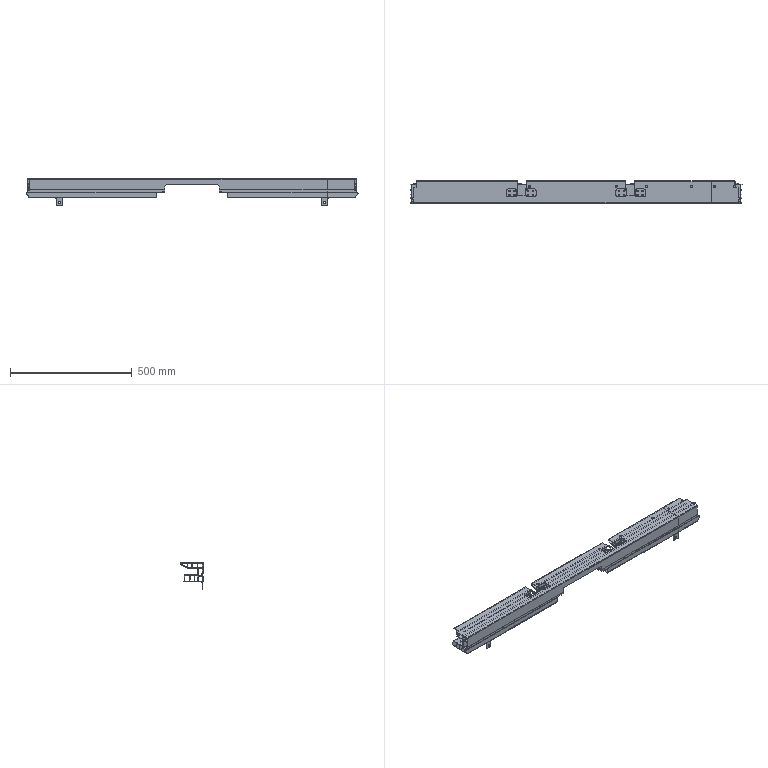NC program | NX | posted with a generic post | part box 1365 x 90.95 x 108.501 mm
Lines 15591 to 16293 of 23380:
(FIXED_CONTOUR_COPY , TOOL : D6)
N31156 T06 M6
N31158 G54
N31160 G17 G0 G90 X-536.513 Y-19.655 B0. C0. S9500 M3
N31162 G43 Z30. H6
N31164 Z-3.359
N31166 G94 G1 Z-8.159 F1000.
N31168 X-536.315 Y-19.457 Z-8.58 F2500.
N31170 X-535.832 Y-18.974 Z-9.536
N31172 X-535.728 Y-18.87 Z-9.73
N31174 X-535.641 Y-18.837 Z-9.891
N31176 X-535.457 Y-18.798 Z-10.212
N31178 X-535.59 Y-18.932 Z-9.981
N31180 X-535.846 Y-19.188 Z-9.51
N31182 X-536.315 Y-19.656 Z-8.576
N31184 X-536.575 Y-19.917 Z-8.023
N31186 X-536.669 Y-20.01 Z-7.818
N31188 X-536.738 Y-20.202 Z-7.664
N31190 X-536.789 Y-20.383 Z-7.549
N31192 X-536.315 Y-19.909 Z-8.572
N31194 X-535.832 Y-19.426 Z-9.539
N31196 X-535.59 Y-19.185 Z-9.982
N31198 X-535.349 Y-18.943 Z-10.392
N31200 X-535.167 Y-18.762 Z-10.649
N31202 X-534.992 Y-18.745 Z-10.887
N31204 X-534.879 Y-18.739 Z-11.039
N31206 X-535.107 Y-18.967 Z-10.728
N31208 X-535.251 Y-19.111 Z-10.528
N31210 X-535.349 Y-19.208 Z-10.389
N31212 X-535.59 Y-19.45 Z-9.983
N31214 X-535.832 Y-19.691 Z-9.538
N31216 X-536.017 Y-19.876 Z-9.168
N31218 X-536.315 Y-20.174 Z-8.564
N31220 X-536.797 Y-20.657 Z-7.521
N31222 X-536.88 Y-20.74 Z-7.338
N31224 X-536.949 Y-21.102 Z-7.178
N31226 X-536.682 Y-20.835 Z-7.76
N31228 X-536.315 Y-20.467 Z-8.554
N31230 X-536.203 Y-20.355 Z-8.785
N31232 X-535.832 Y-19.985 Z-9.538
N31234 X-535.59 Y-19.743 Z-9.986
N31236 X-535.349 Y-19.502 Z-10.388
N31238 X-535.107 Y-19.26 Z-10.729
N31240 X-534.866 Y-19.019 Z-11.056
N31242 X-534.688 Y-18.841 Z-11.269
N31244 X-534.625 Y-18.777 Z-11.349
N31246 X-534.574 Y-18.727 Z-11.406
N31248 X-534.382 Y-18.721 Z-11.611
N31250 X-534.247 Y-18.718 Z-11.745
N31252 X-534.309 Y-18.78 Z-11.682
N31254 X-534.383 Y-18.854 Z-11.61
N31256 X-534.625 Y-19.095 Z-11.344
N31258 X-534.866 Y-19.337 Z-11.056
N31260 X-535.107 Y-19.578 Z-10.731
N31262 X-535.349 Y-19.82 Z-10.39
N31264 X-535.59 Y-20.061 Z-9.988
N31266 X-535.832 Y-20.302 Z-9.536
N31268 X-536.099 Y-20.57 Z-8.992
N31270 X-536.315 Y-20.785 Z-8.541
N31272 X-537. Y-21.47 Z-7.06
N31274 X-537.024 Y-21.668 Z-7.003
N31276 X-537.034 Y-21.829 Z-6.979
N31278 X-536.657 Y-21.453 Z-7.788
N31280 X-536.315 Y-21.11 Z-8.528
N31282 X-536.176 Y-20.972 Z-8.822
N31284 X-535.936 Y-20.731 Z-9.321
N31286 X-535.832 Y-20.628 Z-9.533
N31288 X-535.59 Y-20.386 Z-9.99
N31290 X-535.349 Y-20.145 Z-10.392
N31292 X-535.107 Y-19.903 Z-10.732
N31294 X-534.866 Y-19.662 Z-11.056
N31296 X-534.625 Y-19.42 Z-11.344
N31298 X-534.383 Y-19.179 Z-11.61
N31300 X-534.142 Y-18.938 Z-11.845
N31302 X-533.914 Y-18.71 Z-12.054
N31304 X-533.583 Y-18.705 Z-12.32
N31306 X-533.682 Y-18.804 Z-12.239
N31308 X-533.9 Y-19.022 Z-12.066
N31310 X-534.142 Y-19.264 Z-11.845
N31312 X-534.383 Y-19.505 Z-11.61
N31314 X-534.625 Y-19.747 Z-11.344
N31316 X-534.866 Y-19.988 Z-11.056
N31318 X-535.107 Y-20.23 Z-10.732
N31320 X-535.349 Y-20.471 Z-10.394
N31322 X-535.59 Y-20.712 Z-9.992
N31324 X-535.832 Y-20.954 Z-9.529
N31326 X-536.012 Y-21.135 Z-9.156
N31328 X-536.315 Y-21.437 Z-8.514
N31330 X-536.671 Y-21.793 Z-7.748
N31332 X-537.054 Y-22.176 Z-6.931
N31334 X-537.061 Y-22.509 Z-6.916
N31336 X-536.57 Y-22.019 Z-7.955
N31338 X-536.089 Y-21.538 Z-8.984
N31340 X-535.832 Y-21.28 Z-9.525
N31342 X-535.59 Y-21.039 Z-9.994
N31344 X-535.349 Y-20.797 Z-10.395
N31346 X-535.107 Y-20.556 Z-10.732
N31348 X-534.866 Y-20.314 Z-11.056
N31350 X-534.625 Y-20.073 Z-11.344
N31352 X-534.383 Y-19.831 Z-11.611
N31354 X-534.142 Y-19.59 Z-11.845
N31356 X-533.9 Y-19.349 Z-12.067
N31358 X-533.417 Y-18.866 Z-12.447
N31360 X-533.252 Y-18.7 Z-12.552
N31362 X-532.922 Y-18.696 Z-12.762
N31364 X-533.417 Y-19.192 Z-12.447
N31366 X-533.9 Y-19.675 Z-12.067
N31368 X-534.142 Y-19.916 Z-11.845
N31370 X-534.383 Y-20.158 Z-11.611
N31372 X-534.625 Y-20.399 Z-11.343
N31374 X-534.866 Y-20.64 Z-11.056
N31376 X-535.107 Y-20.882 Z-10.732
N31378 X-535.349 Y-21.123 Z-10.397
N31380 X-535.59 Y-21.365 Z-9.996
N31382 X-535.734 Y-21.508 Z-9.717
N31384 X-535.832 Y-21.606 Z-9.519
N31386 X-536.019 Y-21.793 Z-9.122
N31388 X-536.498 Y-22.272 Z-8.102
N31390 X-537.063 Y-22.837 Z-6.912
N31392 X-537.062 Y-23.162 Z-6.914
N31394 X-536.172 Y-22.272 Z-8.788
N31396 X-535.832 Y-21.932 Z-9.512
N31398 X-535.625 Y-21.725 Z-9.931
N31400 X-535.59 Y-21.691 Z-9.998
N31402 X-535.349 Y-21.449 Z-10.401
N31404 X-535.107 Y-21.208 Z-10.735
N31406 X-534.866 Y-20.967 Z-11.057
N31408 X-534.625 Y-20.725 Z-11.343
N31410 X-534.383 Y-20.484 Z-11.611
N31412 X-534.142 Y-20.242 Z-11.845
N31414 X-533.9 Y-20.001 Z-12.067
N31416 X-533.417 Y-19.518 Z-12.447
N31418 X-532.935 Y-19.035 Z-12.754
N31420 X-532.693 Y-18.794 Z-12.894
N31422 X-532.591 Y-18.692 Z-12.949
N31424 X-532.451 Y-18.689 Z-13.021
N31426 X-532.446 Z-13.025
N31428 X-532.39 Y-18.685 Z-12.995
N31430 X-532.26 Y-18.686 Z-12.925
N31432 X-532.448 Y-18.874 Z-13.023
N31434 X-532.693 Y-19.12 Z-12.893
N31436 X-532.935 Y-19.361 Z-12.754
N31438 X-533.417 Y-19.844 Z-12.447
N31440 X-533.9 Y-20.327 Z-12.067
N31442 X-534.142 Y-20.568 Z-11.845
N31444 X-534.383 Y-20.809 Z-11.611
N31446 X-534.625 Y-21.051 Z-11.345
N31448 X-534.866 Y-21.292 Z-11.06
N31450 X-535.107 Y-21.534 Z-10.741
N31452 X-535.349 Y-21.775 Z-10.409
N31454 X-535.515 Y-21.942 Z-10.133
N31456 X-535.59 Y-22.017 Z-9.993
N31458 X-535.839 Y-22.265 Z-9.489
N31460 X-537.061 Y-23.488 Z-6.916
N31462 Y-23.604 Z-6.917
N31464 X-537.053 Y-23.805 Z-6.936
N31466 X-535.832 Y-22.584 Z-9.502
N31468 X-535.59 Y-22.342 Z-9.986
N31470 X-535.406 Y-22.158 Z-10.329
N31472 X-535.349 Y-22.101 Z-10.424
N31474 X-535.175 Y-21.926 Z-10.659
N31476 X-535.107 Y-21.859 Z-10.753
N31478 X-535.041 Y-21.793 Z-10.835
N31480 X-534.866 Y-21.618 Z-11.066
N31482 X-534.625 Y-21.376 Z-11.348
N31484 X-534.383 Y-21.135 Z-11.613
N31486 X-534.142 Y-20.894 Z-11.845
N31488 X-533.9 Y-20.652 Z-12.067
N31490 X-533.417 Y-20.169 Z-12.447
N31492 X-532.935 Y-19.686 Z-12.754
N31494 X-532.694 Y-19.445 Z-12.894
N31496 X-532.452 Y-19.204 Z-13.024
N31498 X-532.209 Y-18.961 Z-12.893
N31500 X-531.969 Y-18.721 Z-12.754
N31502 X-531.938 Y-18.69 Z-12.735
N31504 X-531.619 Y-18.695 Z-12.532
N31506 X-531.969 Y-19.045 Z-12.754
N31508 X-532.21 Y-19.286 Z-12.894
N31510 X-532.452 Y-19.529 Z-13.024
N31512 X-532.693 Y-19.77 Z-12.894
N31514 X-532.935 Y-20.011 Z-12.754
N31516 X-533.417 Y-20.494 Z-12.447
N31518 X-533.9 Y-20.977 Z-12.068
N31520 X-534.142 Y-21.218 Z-11.847
N31522 X-534.383 Y-21.459 Z-11.616
N31524 X-534.625 Y-21.701 Z-11.353
N31526 X-534.717 Y-21.793 Z-11.246
N31528 X-534.866 Y-21.942 Z-11.085
N31530 X-535.107 Y-22.184 Z-10.78
N31532 X-535.196 Y-22.272 Z-10.657
N31534 X-535.349 Y-22.425 Z-10.432
N31536 X-535.59 Y-22.667 Z-9.985
N31538 X-535.832 Y-22.908 Z-9.501
N31540 X-536.797 Y-23.874 Z-7.474
N31542 X-537.04 Y-24.116 Z-6.969
N31544 X-537.013 Y-24.412 Z-7.035
N31546 X-536.79 Y-24.189 Z-7.495
N31548 X-536.31 Y-23.71 Z-8.496
N31550 X-535.831 Y-23.231 Z-9.502
N31552 X-535.59 Y-22.99 Z-9.985
N31554 X-535.349 Y-22.749 Z-10.432
N31556 X-535.107 Y-22.507 Z-10.787
N31558 X-534.866 Y-22.266 Z-11.118
N31560 X-534.625 Y-22.024 Z-11.379
N31562 X-534.393 Y-21.793 Z-11.609
N31564 X-534.142 Y-21.541 Z-11.85
N31566 X-533.9 Y-21.3 Z-12.069
N31568 X-533.417 Y-20.817 Z-12.447
N31570 X-532.935 Y-20.334 Z-12.754
N31572 X-532.693 Y-20.093 Z-12.894
N31574 X-532.452 Y-19.852 Z-13.024
N31576 X-532.21 Y-19.61 Z-12.894
N31578 X-531.969 Y-19.369 Z-12.754
N31580 X-531.486 Y-18.886 Z-12.447
N31582 X-531.301 Y-18.701 Z-12.305
N31584 X-531.003 Y-18.707 Z-12.066
N31586 X-530.985 Z-12.049
N31588 X-531.003 Y-18.726 Z-12.066
N31590 X-531.486 Y-19.209 Z-12.447
N31592 X-531.969 Y-19.692 Z-12.754
N31594 X-532.21 Y-19.933 Z-12.894
N31596 X-532.451 Y-20.174 Z-13.023
N31598 X-532.693 Y-20.416 Z-12.894
N31600 X-532.935 Y-20.657 Z-12.753
N31602 X-533.417 Y-21.14 Z-12.448
N31604 X-533.9 Y-21.623 Z-12.073
N31606 X-534.07 Y-21.793 Z-11.919
N31608 X-534.383 Y-22.106 Z-11.652
N31610 X-534.55 Y-22.272 Z-11.487
N31612 X-534.625 Y-22.347 Z-11.405
N31614 X-534.866 Y-22.589 Z-11.118
N31616 X-535.107 Y-22.83 Z-10.787
N31618 X-535.349 Y-23.072 Z-10.432
N31620 X-535.59 Y-23.313 Z-9.985
N31622 X-535.832 Y-23.554 Z-9.502
N31624 X-536.797 Y-24.52 Z-7.488
N31626 X-536.978 Y-24.701 Z-7.116
N31628 X-536.936 Y-24.98 Z-7.218
N31630 X-536.797 Y-24.841 Z-7.5
N31632 X-535.832 Y-23.876 Z-9.505
N31634 X-535.59 Y-23.634 Z-9.986
N31636 X-535.349 Y-23.393 Z-10.432
N31638 X-535.107 Y-23.151 Z-10.787
N31640 X-534.866 Y-22.91 Z-11.118
N31642 X-534.625 Y-22.669 Z-11.405
N31644 X-534.383 Y-22.427 Z-11.667
N31646 X-534.228 Y-22.272 Z-11.817
N31648 X-534.138 Y-22.182 Z-11.896
N31650 Z-11.887
N31652 X-534.028 Y-22.072 Z-11.976
N31654 X-533.9 Y-21.944 Z-12.085
N31656 X-533.749 Y-21.793 Z-12.194
N31658 X-533.417 Y-21.461 Z-12.451
N31660 X-532.935 Y-20.979 Z-12.754
N31662 X-532.693 Y-20.737 Z-12.893
N31664 X-532.45 Y-20.495 Z-13.022
N31666 X-532.21 Y-20.254 Z-12.894
N31668 X-531.969 Y-20.013 Z-12.754
N31670 X-531.486 Y-19.53 Z-12.447
N31672 X-531.003 Y-19.047 Z-12.066
N31674 X-530.819 Y-18.863 Z-11.897
N31676 X-530.762 Y-18.806 Z-11.847
N31678 X-530.671 Y-18.715 Z-11.76
N31680 X-530.494 Y-18.72 Z-11.581
N31682 X-530.359 Y-18.724 Z-11.437
N31684 X-530.429 Y-18.794 Z-11.509
N31686 X-530.52 Y-18.886 Z-11.61
N31688 X-530.762 Y-19.127 Z-11.845
N31690 X-531.003 Y-19.368 Z-12.066
N31692 X-531.486 Y-19.851 Z-12.447
N31694 X-531.969 Y-20.334 Z-12.753
N31696 X-532.21 Y-20.575 Z-12.893
N31698 X-532.45 Y-20.815 Z-13.021
N31700 X-532.694 Y-21.059 Z-12.895
N31702 X-532.935 Y-21.3 Z-12.756
N31704 X-533.417 Y-21.783 Z-12.455
N31706 X-533.693 Y-22.058 Z-12.255
N31708 X-533.726 Y-22.091 Z-12.233
N31710 X-533.742 Y-22.108 Z-12.221
N31712 X-533.776 Y-22.141 Z-12.2
N31714 X-533.816 Y-22.181 Z-12.173
N31716 X-533.907 Y-22.272 Z-12.112
N31718 X-534.106 Y-22.471 Z-11.935
N31720 X-534.383 Y-22.748 Z-11.667
N31722 X-534.625 Y-22.99 Z-11.405
N31724 X-534.866 Y-23.231 Z-11.119
N31726 X-535.107 Y-23.473 Z-10.787
N31728 X-535.353 Y-23.718 Z-10.425
N31730 X-535.59 Y-23.956 Z-9.991
N31732 X-535.832 Y-24.197 Z-9.51
N31734 X-536.797 Y-25.163 Z-7.515
N31736 X-536.886 Y-25.251 Z-7.337
N31738 X-536.861 Y-25.378 Z-7.396
N31740 X-536.829 Y-25.511 Z-7.472
N31742 X-536.797 Y-25.479 Z-7.534
N31744 X-536.466 Y-25.148 Z-8.212
N31746 X-536.315 Y-24.996 Z-8.526
N31748 X-535.832 Y-24.513 Z-9.516
N31750 X-535.723 Y-24.405 Z-9.726
N31752 X-535.59 Y-24.272 Z-9.995
N31754 X-535.349 Y-24.03 Z-10.419
N31756 X-535.242 Y-23.923 Z-10.573
N31758 X-535.107 Y-23.789 Z-10.781
N31760 X-535.029 Y-23.71 Z-10.895
N31762 X-534.866 Y-23.547 Z-11.118
N31764 X-534.625 Y-23.306 Z-11.405
N31766 X-534.383 Y-23.065 Z-11.667
N31768 X-534.142 Y-22.823 Z-11.901
N31770 X-533.9 Y-22.582 Z-12.118
N31772 X-533.591 Y-22.272 Z-12.36
N31774 X-533.452 Y-22.134 Z-12.45
N31776 X-533.417 Y-22.099 Z-12.473
N31778 X-533.351 Y-22.033 Z-12.51
N31780 X-533.112 Y-21.793 Z-12.651
N31782 X-532.935 Y-21.616 Z-12.762
N31784 X-532.694 Y-21.376 Z-12.898
N31786 X-532.453 Y-21.134 Z-13.023
N31788 X-532.21 Y-20.891 Z-12.893
N31790 X-531.969 Y-20.65 Z-12.753
N31792 X-531.486 Y-20.167 Z-12.447
N31794 X-531.003 Y-19.685 Z-12.066
N31796 X-530.762 Y-19.443 Z-11.844
N31798 X-530.52 Y-19.202 Z-11.61
N31800 X-530.279 Y-18.96 Z-11.344
N31802 X-530.055 Y-18.737 Z-11.077
N31804 X-529.905 Y-18.745 Z-10.878
N31806 X-529.778 Y-18.757 Z-10.707
N31808 X-529.878 Y-18.857 Z-10.836
N31810 X-530.037 Y-19.016 Z-11.056
N31812 X-530.279 Y-19.258 Z-11.344
N31814 X-530.52 Y-19.499 Z-11.61
N31816 X-530.762 Y-19.741 Z-11.844
N31818 X-531.003 Y-19.982 Z-12.067
N31820 X-531.486 Y-20.465 Z-12.447
N31822 X-531.969 Y-20.948 Z-12.754
N31824 X-532.21 Y-21.189 Z-12.895
N31826 X-532.454 Y-21.433 Z-13.026
N31828 X-532.694 Y-21.673 Z-12.902
N31830 X-532.814 Y-21.793 Z-12.835
N31832 X-532.935 Y-21.913 Z-12.771
N31834 X-533.113 Y-22.092 Z-12.668
N31836 X-533.293 Y-22.272 Z-12.572
N31838 X-533.417 Y-22.396 Z-12.493
N31840 X-533.659 Y-22.638 Z-12.308
N31842 X-533.9 Y-22.879 Z-12.118
N31844 X-534.142 Y-23.121 Z-11.901
N31846 X-534.383 Y-23.362 Z-11.667
N31848 X-534.625 Y-23.603 Z-11.405
N31850 X-534.731 Y-23.71 Z-11.279
N31852 X-534.798 Y-23.777 Z-11.189
N31854 X-534.821 Y-23.8 Z-11.163
N31856 X-534.866 Y-23.845 Z-11.106
N31858 X-534.981 Y-23.96 Z-10.937
N31860 X-535.107 Y-24.086 Z-10.758
N31862 X-535.142 Y-24.121 Z-10.705
N31864 X-535.349 Y-24.328 Z-10.408
N31866 X-535.59 Y-24.569 Z-9.993
N31868 X-535.784 Y-24.763 Z-9.611
N31870 X-535.832 Y-24.811 Z-9.521
N31872 X-536.169 Y-25.148 Z-8.832
N31874 X-536.315 Y-25.293 Z-8.538
N31876 X-536.762 Y-25.741 Z-7.624
N31878 X-536.747 Y-25.792 Z-7.659
N31880 X-536.687 Y-25.958 Z-7.793
N31882 X-536.315 Y-25.586 Z-8.55
N31884 X-535.832 Y-25.103 Z-9.525
N31886 X-535.686 Y-24.957 Z-9.803
N31888 X-535.59 Y-24.862 Z-9.991
N31890 X-535.526 Y-24.797 Z-10.098
N31892 X-535.349 Y-24.62 Z-10.4
N31894 X-535.107 Y-24.379 Z-10.745
N31896 X-534.883 Y-24.155 Z-11.053
N31898 X-534.866 Y-24.137 Z-11.078
N31900 X-534.723 Y-23.994 Z-11.26
N31902 X-534.652 Y-23.923 Z-11.342
N31904 X-534.562 Y-23.834 Z-11.461
N31906 X-534.439 Y-23.71 Z-11.607
N31908 X-534.383 Y-23.655 Z-11.667
N31910 X-534.142 Y-23.413 Z-11.901
N31912 X-533.9 Y-23.172 Z-12.118
N31914 X-533.48 Y-22.752 Z-12.447
N31916 X-533.417 Y-22.689 Z-12.495
N31918 X-533.001 Y-22.272 Z-12.758
N31920 X-532.935 Y-22.206 Z-12.794
N31922 X-532.821 Y-22.092 Z-12.847
N31924 X-532.695 Y-21.966 Z-12.912
N31926 X-532.522 Y-21.793 Z-12.995
N31928 X-532.454 Y-21.725 Z-13.03
N31930 X-532.21 Y-21.482 Z-12.898
N31932 X-531.969 Y-21.24 Z-12.756
N31934 X-531.486 Y-20.757 Z-12.447
N31936 X-531.003 Y-20.275 Z-12.067
N31938 X-530.762 Y-20.033 Z-11.844
N31940 X-530.52 Y-19.792 Z-11.61
N31942 X-530.279 Y-19.55 Z-11.343
N31944 X-530.037 Y-19.309 Z-11.056
N31946 X-529.906 Y-19.178 Z-10.878
N31948 X-529.746 Y-19.017 Z-10.654
N31950 X-529.646 Y-18.918 Z-10.512
N31952 X-529.585 Y-18.857 Z-10.428
N31954 X-529.514 Y-18.785 Z-10.311
N31956 X-529.313 Y-18.826 Z-9.987
N31958 X-529.276 Y-18.834 Z-9.918
N31960 X-529.313 Y-18.872 Z-9.983
N31962 X-529.359 Y-18.918 Z-10.056
N31964 X-529.555 Y-19.113 Z-10.384
N31966 X-529.81 Y-19.369 Z-10.748
N31968 X-530.037 Y-19.596 Z-11.056
N31970 X-530.279 Y-19.837 Z-11.343
N31972 X-530.52 Y-20.079 Z-11.61
N31974 X-530.762 Y-20.32 Z-11.844
N31976 X-531.003 Y-20.562 Z-12.067
N31978 X-531.486 Y-21.045 Z-12.448
N31980 X-531.969 Y-21.527 Z-12.759
N31982 X-532.235 Y-21.793 Z-12.915
N31984 X-532.455 Y-22.013 Z-13.041
N31986 X-532.534 Y-22.092 Z-13.003
N31988 X-532.714 Y-22.272 Z-12.923
N31990 X-532.935 Y-22.493 Z-12.801
N31992 X-533.417 Y-22.976 Z-12.495
N31994 X-533.9 Y-23.459 Z-12.118
N31996 X-534.152 Y-23.71 Z-11.891
N31998 X-534.188 Y-23.746 Z-11.846
N32000 X-534.228 Y-23.787 Z-11.803
N32002 X-534.306 Y-23.864 Z-11.727
N32004 X-534.383 Y-23.942 Z-11.645
N32006 X-534.466 Y-24.025 Z-11.547
N32008 X-534.507 Y-24.066 Z-11.492
N32010 X-534.631 Y-24.189 Z-11.35
N32012 X-534.866 Y-24.425 Z-11.067
N32014 X-535.107 Y-24.666 Z-10.737
N32016 X-535.349 Y-24.907 Z-10.393
N32018 X-535.429 Y-24.988 Z-10.255
N32020 X-535.59 Y-25.148 Z-9.99
N32022 X-535.75 Y-25.309 Z-9.681
N32024 X-535.832 Y-25.39 Z-9.529
N32026 X-536.191 Y-25.75 Z-8.802
N32028 X-536.315 Y-25.873 Z-8.559
N32030 X-536.604 Y-26.163 Z-7.975
N32032 X-536.552 Y-26.286 Z-8.092
N32034 X-536.509 Y-26.36 Z-8.181
N32036 X-536.045 Y-25.895 Z-9.1
N32038 X-535.832 Y-25.682 Z-9.532
N32040 X-535.653 Y-25.503 Z-9.867
N32042 X-535.59 Y-25.441 Z-9.987
N32044 X-535.349 Y-25.199 Z-10.387
N32046 X-535.107 Y-24.958 Z-10.732
N32048 X-535.01 Y-24.861 Z-10.865
N32050 X-534.866 Y-24.717 Z-11.06
N32052 X-534.625 Y-24.475 Z-11.351
N32054 X-534.383 Y-24.234 Z-11.621
N32056 X-534.339 Y-24.189 Z-11.664
N32058 X-534.208 Y-24.058 Z-11.803
N32060 X-534.002 Y-23.852 Z-12.007
N32062 X-533.9 Y-23.751 Z-12.115
N32064 X-533.877 Y-23.728 Z-12.136
N32066 X-533.417 Y-23.268 Z-12.495
N32068 X-532.935 Y-22.785 Z-12.801
N32070 X-532.693 Y-22.544 Z-12.934
N32072 X-532.453 Y-22.303 Z-13.054
N32074 X-532.398 Y-22.248 Z-13.023
N32076 X-532.21 Y-22.061 Z-12.914
N32078 X-532.076 Y-21.926 Z-12.831
N32080 X-531.943 Y-21.793 Z-12.746
N32082 X-531.486 Y-21.337 Z-12.449
N32084 X-531.003 Y-20.854 Z-12.067
N32086 X-530.762 Y-20.612 Z-11.845
N32088 X-530.52 Y-20.371 Z-11.61
N32090 X-530.279 Y-20.129 Z-11.343
N32092 X-530.037 Y-19.888 Z-11.056
N32094 X-529.796 Y-19.647 Z-10.729
N32096 X-529.555 Y-19.405 Z-10.387
N32098 X-529.313 Y-19.164 Z-9.979
N32100 X-529.061 Y-18.912 Z-9.522
N32102 X-528.909 Y-18.973 Z-9.227
N32104 X-528.864 Y-19.018 Z-9.139
N32106 X-529.072 Y-19.226 Z-9.537
N32108 X-529.313 Y-19.468 Z-9.979
N32110 X-529.555 Y-19.709 Z-10.387
N32112 X-529.796 Y-19.951 Z-10.729
N32114 X-530.037 Y-20.192 Z-11.056
N32116 X-530.279 Y-20.433 Z-11.343
N32118 X-530.52 Y-20.675 Z-11.611
N32120 X-530.762 Y-20.916 Z-11.845
N32122 X-531.003 Y-21.158 Z-12.068
N32124 X-531.486 Y-21.641 Z-12.453
N32126 X-531.639 Y-21.793 Z-12.552
N32128 X-531.786 Y-21.94 Z-12.656
N32130 X-531.803 Y-21.958 Z-12.669
N32132 X-531.934 Y-22.088 Z-12.757
N32134 X-532.01 Y-22.164 Z-12.809
N32136 X-532.118 Y-22.272 Z-12.879
N32138 X-532.34 Y-22.494 Z-12.998
N32140 X-532.452 Y-22.607 Z-13.054
N32142 X-532.693 Y-22.848 Z-12.934
N32144 X-532.935 Y-23.089 Z-12.801
N32146 X-533.417 Y-23.572 Z-12.494
N32148 X-533.574 Y-23.728 Z-12.373
N32150 X-533.601 Y-23.755 Z-12.346
N32152 X-533.646 Y-23.8 Z-12.309
N32154 X-533.698 Y-23.852 Z-12.259
N32156 X-533.761 Y-23.915 Z-12.205
N32158 X-533.83 Y-23.985 Z-12.144
N32160 X-533.9 Y-24.055 Z-12.084
N32162 X-534.035 Y-24.189 Z-11.952
N32164 X-534.142 Y-24.296 Z-11.853
N32166 X-534.383 Y-24.538 Z-11.616
N32168 X-534.625 Y-24.779 Z-11.345
N32170 X-534.866 Y-25.02 Z-11.057
N32172 X-535.107 Y-25.262 Z-10.728
N32174 X-535.349 Y-25.503 Z-10.386
N32176 X-535.59 Y-25.745 Z-9.984
N32178 X-535.711 Y-25.866 Z-9.755
N32180 X-535.832 Y-25.986 Z-9.532
N32182 X-535.952 Y-26.106 Z-9.292
N32184 X-536.399 Y-26.553 Z-8.416
N32186 X-536.371 Y-26.602 Z-8.475
N32188 X-536.262 Y-26.734 Z-8.698
N32190 X-536.113 Y-26.585 Z-8.983
N32192 X-535.832 Y-26.304 Z-9.533
N32194 X-535.59 Y-26.063 Z-9.981
N32196 X-535.444 Y-25.917 Z-10.228
N32198 X-535.349 Y-25.821 Z-10.386
N32200 X-535.107 Y-25.58 Z-10.729
N32202 X-534.866 Y-25.338 Z-11.056
N32204 X-534.625 Y-25.097 Z-11.343
N32206 X-534.383 Y-24.856 Z-11.613
N32208 X-534.142 Y-24.614 Z-11.848
N32210 X-533.9 Y-24.373 Z-12.073
N32212 X-533.717 Y-24.189 Z-12.22
N32214 X-533.417 Y-23.89 Z-12.473
N32216 X-533.238 Y-23.71 Z-12.607
N32218 X-532.935 Y-23.407 Z-12.8
N32220 X-532.876 Y-23.348 Z-12.831
N32222 X-532.693 Y-23.166 Z-12.934
N32224 X-532.452 Y-22.924 Z-13.054
N32226 X-532.21 Y-22.683 Z-12.933
N32228 X-531.969 Y-22.441 Z-12.799
N32230 X-531.8 Y-22.272 Z-12.691
N32232 X-531.696 Y-22.168 Z-12.614
N32234 X-531.644 Y-22.116 Z-12.58
N32236 X-531.568 Y-22.04 Z-12.521
N32238 X-531.486 Y-21.958 Z-12.464
N32240 X-531.321 Y-21.793 Z-12.325
N32242 X-531.003 Y-21.476 Z-12.071
N32244 X-530.762 Y-21.234 Z-11.847
N32246 X-530.52 Y-20.993 Z-11.612
N32248 X-530.279 Y-20.751 Z-11.343
N32250 X-530.037 Y-20.51 Z-11.056
N32252 X-529.796 Y-20.268 Z-10.729
N32254 X-529.555 Y-20.027 Z-10.386
N32256 X-529.313 Y-19.786 Z-9.98
N32258 X-529.072 Y-19.544 Z-9.533
N32260 X-528.89 Y-19.362 Z-9.18
N32262 X-528.708 Y-19.181 Z-8.831
N32264 X-528.661 Y-19.23 Z-8.737
N32266 X-528.565 Y-19.357 Z-8.543
N32268 X-529.072 Y-19.864 Z-9.532
N32270 X-529.313 Y-20.105 Z-9.983
N32272 X-529.397 Y-20.189 Z-10.124
N32274 X-529.555 Y-20.347 Z-10.386
N32276 X-529.796 Y-20.588 Z-10.728
N32278 X-530.037 Y-20.83 Z-11.056
N32280 X-530.279 Y-21.071 Z-11.344
N32282 X-530.52 Y-21.312 Z-11.614
N32284 X-530.762 Y-21.554 Z-11.85
N32286 X-531.003 Y-21.795 Z-12.075
N32288 X-531.367 Y-22.159 Z-12.386
N32290 X-531.486 Y-22.278 Z-12.491
N32292 X-531.969 Y-22.761 Z-12.801
N32294 X-532.21 Y-23.002 Z-12.934
N32296 X-532.452 Y-23.244 Z-13.054
N32298 X-532.693 Y-23.485 Z-12.93
N32300 X-532.769 Y-23.561 Z-12.887
N32302 X-532.918 Y-23.71 Z-12.808
N32304 X-532.935 Y-23.727 Z-12.797
N32306 X-533.158 Y-23.95 Z-12.633
N32308 X-533.417 Y-24.209 Z-12.455
N32310 X-533.9 Y-24.692 Z-12.069
N32312 X-534.142 Y-24.934 Z-11.846
N32314 X-534.383 Y-25.175 Z-11.611
N32316 X-534.625 Y-25.417 Z-11.343
N32318 X-534.866 Y-25.658 Z-11.056
N32320 X-535.107 Y-25.899 Z-10.729
N32322 X-535.349 Y-26.141 Z-10.387
N32324 X-535.59 Y-26.382 Z-9.98
N32326 X-535.838 Y-26.63 Z-9.523
N32328 X-536.108 Y-26.9 Z-9.004
N32330 X-535.961 Y-27.042 Z-9.296
N32332 X-535.938 Y-27.051 Z-9.34
N32334 X-535.832 Y-26.945 Z-9.54
N32336 X-535.59 Y-26.704 Z-9.979
N32338 X-535.349 Y-26.462 Z-10.387
N32340 X-535.107 Y-26.221 Z-10.729
N32342 X-534.866 Y-25.98 Z-11.056
N32344 X-534.625 Y-25.738 Z-11.343
N32346 X-534.383 Y-25.497 Z-11.611
N32348 X-534.142 Y-25.255 Z-11.845
N32350 X-533.9 Y-25.014 Z-12.068
N32352 X-533.417 Y-24.531 Z-12.451
N32354 X-533.076 Y-24.189 Z-12.671
N32356 X-532.935 Y-24.048 Z-12.768
N32358 X-532.693 Y-23.807 Z-12.92
N32360 X-532.597 Y-23.71 Z-12.974
N32362 X-532.452 Y-23.565 Z-13.048
N32364 X-532.21 Y-23.324 Z-12.932
N32366 X-531.969 Y-23.082 Z-12.801
N32368 X-531.486 Y-22.6 Z-12.494
N32370 X-531.159 Y-22.272 Z-12.24
N32372 X-531.003 Y-22.117 Z-12.099
N32374 X-530.961 Y-22.075 Z-12.057
N32376 X-530.947 Y-22.061 Z-12.041
N32378 X-530.734 Y-21.848 Z-11.832
N32380 X-530.68 Y-21.793 Z-11.774
N32382 X-530.52 Y-21.634 Z-11.618
N32384 X-530.279 Y-21.392 Z-11.347
N32386 X-530.037 Y-21.151 Z-11.058
N32388 X-529.932 Y-21.045 Z-10.916
N32390 X-529.771 Y-20.884 Z-10.694
N32392 X-529.555 Y-20.668 Z-10.386
N32394 X-529.313 Y-20.427 Z-9.986
N32396 X-529.072 Y-20.185 Z-9.532
N32398 X-528.891 Y-20.005 Z-9.167
N32400 X-528.565 Y-19.678 Z-8.526
N32402 X-528.443 Y-19.556 Z-8.284
N32404 X-528.347 Y-19.72 Z-8.082
N32406 X-528.329 Y-19.764 Z-8.041
N32408 X-528.441 Y-19.876 Z-8.263
N32410 X-528.589 Y-20.024 Z-8.561
N32412 X-528.755 Y-20.19 Z-8.89
N32414 X-529.072 Y-20.507 Z-9.53
N32416 X-529.182 Y-20.617 Z-9.735
N32418 X-529.313 Y-20.748 Z-9.989
N32420 X-529.503 Y-20.938 Z-10.301
N32422 X-529.555 Y-20.99 Z-10.39
N32424 X-529.824 Y-21.259 Z-10.773
N32426 X-530.037 Y-21.473 Z-11.064
N32428 X-530.279 Y-21.714 Z-11.354
N32430 X-530.439 Y-21.874 Z-11.536
N32432 X-530.466 Y-21.901 Z-11.572
N32434 X-530.52 Y-21.955 Z-11.636
N32436 X-530.627 Y-22.062 Z-11.749
N32438 X-530.732 Y-22.167 Z-11.852
N32440 X-530.805 Y-22.24 Z-11.935
N32442 X-530.837 Y-22.272 Z-11.968
N32444 X-531.003 Y-22.438 Z-12.118
N32446 X-531.486 Y-22.921 Z-12.495
N32448 X-531.969 Y-23.404 Z-12.8
N32450 X-532.21 Y-23.645 Z-12.927
N32452 X-532.275 Y-23.71 Z-12.958
N32454 X-532.452 Y-23.887 Z-13.035
N32456 X-532.693 Y-24.128 Z-12.9
N32458 X-532.754 Y-24.189 Z-12.862
N32460 X-532.935 Y-24.37 Z-12.759
N32462 X-533.417 Y-24.852 Z-12.448
N32464 X-533.9 Y-25.335 Z-12.067
N32466 X-534.142 Y-25.577 Z-11.845
N32468 X-534.383 Y-25.818 Z-11.61
N32470 X-534.625 Y-26.06 Z-11.343
N32472 X-534.866 Y-26.301 Z-11.056
N32474 X-535.107 Y-26.542 Z-10.729
N32476 X-535.349 Y-26.784 Z-10.385
N32478 X-535.59 Y-27.025 Z-9.98
N32480 X-535.705 Y-27.14 Z-9.777
N32482 X-535.642 Y-27.163 Z-9.892
N32484 X-535.59 Y-27.175 Z-9.988
N32486 X-535.449 Y-27.204 Z-10.216
N32488 X-535.423 Y-27.178 Z-10.256
N32490 X-535.349 Y-27.104 Z-10.381
N32492 X-535.107 Y-26.863 Z-10.727
N32494 X-535.015 Y-26.77 Z-10.855
N32496 X-534.866 Y-26.621 Z-11.056
N32498 X-534.625 Y-26.38 Z-11.343
N32500 X-534.383 Y-26.138 Z-11.61
N32502 X-534.142 Y-25.897 Z-11.844
N32504 X-533.9 Y-25.655 Z-12.067
N32506 X-533.417 Y-25.173 Z-12.447
N32508 X-532.935 Y-24.69 Z-12.755
N32510 X-532.693 Y-24.448 Z-12.893
N32512 X-532.452 Y-24.207 Z-13.016
N32514 X-532.21 Y-23.965 Z-12.91
N32516 X-532.082 Y-23.837 Z-12.845
N32518 X-531.969 Y-23.724 Z-12.797
N32520 X-531.955 Y-23.71 Z-12.79
N32522 X-531.486 Y-23.241 Z-12.495
N32524 X-531.003 Y-22.758 Z-12.118
N32526 X-530.762 Y-22.517 Z-11.9
N32528 X-530.517 Y-22.272 Z-11.663
N32530 X-530.359 Y-22.114 Z-11.476
N32532 X-530.278 Y-22.033 Z-11.369
N32534 X-530.198 Y-21.953 Z-11.276
N32536 X-530.037 Y-21.793 Z-11.072
N32538 X-529.796 Y-21.551 Z-10.743
N32540 X-529.555 Y-21.31 Z-10.398
N32542 X-529.395 Y-21.151 Z-10.126
N32544 X-529.313 Y-21.068 Z-9.99
N32546 X-529.235 Y-20.99 Z-9.837
N32548 X-529.072 Y-20.827 Z-9.526
N32550 X-528.589 Y-20.344 Z-8.552
N32552 X-528.338 Y-20.093 Z-8.04
N32554 X-528.236 Y-19.991 Z-7.834